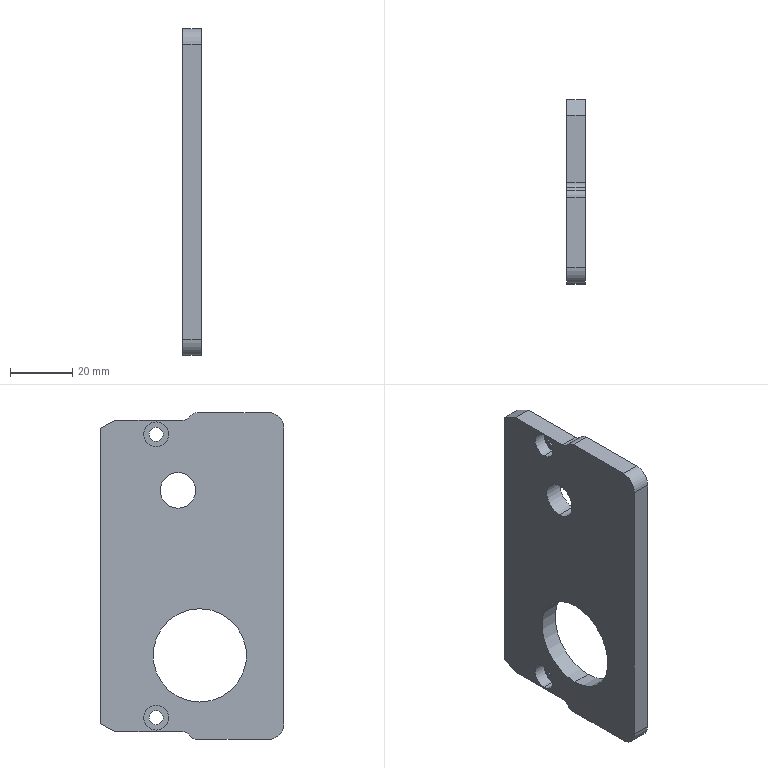Part | SolidWorks | features BaseBody 1 | 1 solid | 32 faces | box 6 x 59 x 105 mm | volume 30844 mm3 | cylinder 18 | plane 14 | commonest cylinder face diameters 4.5 x4 8 x4 5 x3 10 x2 11.445 x2 30 x2
STEP:
#1=CARTESIAN_POINT('',(-288.521,1920.544,-115.75));
#2=VERTEX_POINT('',#1);
#3=CARTESIAN_POINT('',(-288.521,1920.544,-120.25));
#4=VERTEX_POINT('',#3);
#5=CARTESIAN_POINT('',(-288.521,1920.544,-118.));
#6=DIRECTION('',(1.,0.,0.));
#7=DIRECTION('',(0.,0.,1.));
#8=AXIS2_PLACEMENT_3D('',#5,#6,#7);
#9=CIRCLE('',#8,2.25);
#10=EDGE_CURVE('',#2,#4,#9,.T.);
#11=ORIENTED_EDGE('',*,*,#10,.T.);
#12=CARTESIAN_POINT('',(-290.521,1920.544,-120.25));
#13=VERTEX_POINT('',#12);
#14=CARTESIAN_POINT('',(-173.931,1920.544,-120.25));
#15=DIRECTION('',(-1.,0.,0.));
#16=VECTOR('',#15,1000.);
#17=LINE('',#14,#16);
#18=EDGE_CURVE('',#4,#13,#17,.T.);
#19=ORIENTED_EDGE('',*,*,#18,.T.);
#20=CARTESIAN_POINT('',(-290.521,1920.544,-115.75));
#21=VERTEX_POINT('',#20);
#22=CARTESIAN_POINT('',(-290.521,1920.544,-118.));
#23=DIRECTION('',(1.,0.,0.));
#24=DIRECTION('',(0.,0.,1.));
#25=AXIS2_PLACEMENT_3D('',#22,#23,#24);
#26=CIRCLE('',#25,2.25);
#27=EDGE_CURVE('',#21,#13,#26,.T.);
#28=ORIENTED_EDGE('',*,*,#27,.F.);
#29=CARTESIAN_POINT('',(-173.931,1920.544,-115.75));
#30=DIRECTION('',(-1.,0.,0.));
#31=VECTOR('',#30,1000.);
#32=LINE('',#29,#31);
#33=EDGE_CURVE('',#2,#21,#32,.T.);
#34=ORIENTED_EDGE('',*,*,#33,.F.);
#35=EDGE_LOOP('',(#11,#19,#28,#34));
#36=FACE_OUTER_BOUND('',#35,.T.);
#37=CARTESIAN_POINT('',(-173.931,1920.544,-118.));
#38=DIRECTION('',(-1.,0.,0.));
#39=DIRECTION('',(0.,0.,1.));
#40=AXIS2_PLACEMENT_3D('',#37,#38,#39);
#41=CYLINDRICAL_SURFACE('',#40,2.25);
#42=ADVANCED_FACE('',(#36),#41,.F.);
#43=CARTESIAN_POINT('',(-288.521,1913.544,-39.278));
#44=VERTEX_POINT('',#43);
#45=CARTESIAN_POINT('',(-288.521,1913.544,-50.723));
#46=VERTEX_POINT('',#45);
#47=CARTESIAN_POINT('',(-288.521,1913.544,-45.));
#48=DIRECTION('',(1.,0.,0.));
#49=DIRECTION('',(0.,0.,1.));
#50=AXIS2_PLACEMENT_3D('',#47,#48,#49);
#51=CIRCLE('',#50,5.722);
#52=EDGE_CURVE('',#44,#46,#51,.T.);
#53=ORIENTED_EDGE('',*,*,#52,.T.);
#54=CARTESIAN_POINT('',(-294.521,1913.544,-50.723));
#55=VERTEX_POINT('',#54);
#56=CARTESIAN_POINT('',(-290.521,1913.544,-50.723));
#57=DIRECTION('',(-1.,0.,0.));
#58=VECTOR('',#57,1000.);
#59=LINE('',#56,#58);
#60=EDGE_CURVE('',#46,#55,#59,.T.);
#61=ORIENTED_EDGE('',*,*,#60,.T.);
#62=CARTESIAN_POINT('',(-294.521,1913.544,-39.278));
#63=VERTEX_POINT('',#62);
#64=CARTESIAN_POINT('',(-294.521,1913.544,-45.));
#65=DIRECTION('',(1.,0.,0.));
#66=DIRECTION('',(0.,0.,1.));
#67=AXIS2_PLACEMENT_3D('',#64,#65,#66);
#68=CIRCLE('',#67,5.722);
#69=EDGE_CURVE('',#63,#55,#68,.T.);
#70=ORIENTED_EDGE('',*,*,#69,.F.);
#71=CARTESIAN_POINT('',(-290.521,1913.544,-39.278));
#72=DIRECTION('',(-1.,0.,0.));
#73=VECTOR('',#72,1000.);
#74=LINE('',#71,#73);
#75=EDGE_CURVE('',#44,#63,#74,.T.);
#76=ORIENTED_EDGE('',*,*,#75,.F.);
#77=EDGE_LOOP('',(#53,#61,#70,#76));
#78=FACE_OUTER_BOUND('',#77,.T.);
#79=CARTESIAN_POINT('',(-290.521,1913.544,-45.));
#80=DIRECTION('',(-1.,0.,0.));
#81=DIRECTION('',(0.,0.,1.));
#82=AXIS2_PLACEMENT_3D('',#79,#80,#81);
#83=CYLINDRICAL_SURFACE('',#82,5.722);
#84=ADVANCED_FACE('',(#78),#83,.F.);
#85=CARTESIAN_POINT('',(-288.521,1906.544,-83.));
#86=VERTEX_POINT('',#85);
#87=CARTESIAN_POINT('',(-288.521,1906.544,-113.));
#88=VERTEX_POINT('',#87);
#89=CARTESIAN_POINT('',(-288.521,1906.544,-98.));
#90=DIRECTION('',(1.,0.,0.));
#91=DIRECTION('',(0.,0.,1.));
#92=AXIS2_PLACEMENT_3D('',#89,#90,#91);
#93=CIRCLE('',#92,15.);
#94=EDGE_CURVE('',#86,#88,#93,.T.);
#95=ORIENTED_EDGE('',*,*,#94,.T.);
#96=CARTESIAN_POINT('',(-294.521,1906.544,-113.));
#97=VERTEX_POINT('',#96);
#98=CARTESIAN_POINT('',(-173.931,1906.544,-113.));
#99=DIRECTION('',(-1.,0.,0.));
#100=VECTOR('',#99,1000.);
#101=LINE('',#98,#100);
#102=EDGE_CURVE('',#88,#97,#101,.T.);
#103=ORIENTED_EDGE('',*,*,#102,.T.);
#104=CARTESIAN_POINT('',(-294.521,1906.544,-83.));
#105=VERTEX_POINT('',#104);
#106=CARTESIAN_POINT('',(-294.521,1906.544,-98.));
#107=DIRECTION('',(1.,0.,0.));
#108=DIRECTION('',(0.,0.,1.));
#109=AXIS2_PLACEMENT_3D('',#106,#107,#108);
#110=CIRCLE('',#109,15.);
#111=EDGE_CURVE('',#105,#97,#110,.T.);
#112=ORIENTED_EDGE('',*,*,#111,.F.);
#113=CARTESIAN_POINT('',(-173.931,1906.544,-83.));
#114=DIRECTION('',(-1.,0.,0.));
#115=VECTOR('',#114,1000.);
#116=LINE('',#113,#115);
#117=EDGE_CURVE('',#86,#105,#116,.T.);
#118=ORIENTED_EDGE('',*,*,#117,.F.);
#119=EDGE_LOOP('',(#95,#103,#112,#118));
#120=FACE_OUTER_BOUND('',#119,.T.);
#121=CARTESIAN_POINT('',(-173.931,1906.544,-98.));
#122=DIRECTION('',(-1.,0.,0.));
#123=DIRECTION('',(0.,0.,1.));
#124=AXIS2_PLACEMENT_3D('',#121,#122,#123);
#125=CYLINDRICAL_SURFACE('',#124,15.);
#126=ADVANCED_FACE('',(#120),#125,.F.);
#127=CARTESIAN_POINT('',(-288.521,1920.544,-24.75));
#128=VERTEX_POINT('',#127);
#129=CARTESIAN_POINT('',(-288.521,1920.544,-29.25));
#130=VERTEX_POINT('',#129);
#131=CARTESIAN_POINT('',(-288.521,1920.544,-27.));
#132=DIRECTION('',(1.,0.,0.));
#133=DIRECTION('',(0.,0.,1.));
#134=AXIS2_PLACEMENT_3D('',#131,#132,#133);
#135=CIRCLE('',#134,2.25);
#136=EDGE_CURVE('',#128,#130,#135,.T.);
#137=ORIENTED_EDGE('',*,*,#136,.T.);
#138=CARTESIAN_POINT('',(-290.521,1920.544,-29.25));
#139=VERTEX_POINT('',#138);
#140=CARTESIAN_POINT('',(-173.931,1920.544,-29.25));
#141=DIRECTION('',(-1.,0.,0.));
#142=VECTOR('',#141,1000.);
#143=LINE('',#140,#142);
#144=EDGE_CURVE('',#130,#139,#143,.T.);
#145=ORIENTED_EDGE('',*,*,#144,.T.);
#146=CARTESIAN_POINT('',(-290.521,1920.544,-24.75));
#147=VERTEX_POINT('',#146);
#148=CARTESIAN_POINT('',(-290.521,1920.544,-27.));
#149=DIRECTION('',(1.,0.,0.));
#150=DIRECTION('',(0.,0.,1.));
#151=AXIS2_PLACEMENT_3D('',#148,#149,#150);
#152=CIRCLE('',#151,2.25);
#153=EDGE_CURVE('',#147,#139,#152,.T.);
#154=ORIENTED_EDGE('',*,*,#153,.F.);
#155=CARTESIAN_POINT('',(-173.931,1920.544,-24.75));
#156=DIRECTION('',(-1.,0.,0.));
#157=VECTOR('',#156,1000.);
#158=LINE('',#155,#157);
#159=EDGE_CURVE('',#128,#147,#158,.T.);
#160=ORIENTED_EDGE('',*,*,#159,.F.);
#161=EDGE_LOOP('',(#137,#145,#154,#160));
#162=FACE_OUTER_BOUND('',#161,.T.);
#163=CARTESIAN_POINT('',(-173.931,1920.544,-27.));
#164=DIRECTION('',(-1.,0.,0.));
#165=DIRECTION('',(0.,0.,1.));
#166=AXIS2_PLACEMENT_3D('',#163,#164,#165);
#167=CYLINDRICAL_SURFACE('',#166,2.25);
#168=ADVANCED_FACE('',(#162),#167,.F.);
#169=CARTESIAN_POINT('',(-290.521,1920.544,-122.));
#170=VERTEX_POINT('',#169);
#171=CARTESIAN_POINT('',(-290.521,1920.544,-114.));
#172=VERTEX_POINT('',#171);
#173=CARTESIAN_POINT('',(-290.521,1920.544,-118.));
#174=DIRECTION('',(-1.,0.,0.));
#175=DIRECTION('',(0.,0.,1.));
#176=AXIS2_PLACEMENT_3D('',#173,#174,#175);
#177=CIRCLE('',#176,4.);
#178=EDGE_CURVE('',#170,#172,#177,.T.);
#179=ORIENTED_EDGE('',*,*,#178,.F.);
#180=CARTESIAN_POINT('',(-294.521,1920.544,-122.));
#181=VERTEX_POINT('',#180);
#182=CARTESIAN_POINT('',(-292.521,1920.544,-122.));
#183=DIRECTION('',(-1.,0.,0.));
#184=VECTOR('',#183,1000.);
#185=LINE('',#182,#184);
#186=EDGE_CURVE('',#170,#181,#185,.T.);
#187=ORIENTED_EDGE('',*,*,#186,.T.);
#188=CARTESIAN_POINT('',(-294.521,1920.544,-114.));
#189=VERTEX_POINT('',#188);
#190=CARTESIAN_POINT('',(-294.521,1920.544,-118.));
#191=DIRECTION('',(1.,0.,0.));
#192=DIRECTION('',(0.,0.,1.));
#193=AXIS2_PLACEMENT_3D('',#190,#191,#192);
#194=CIRCLE('',#193,4.);
#195=EDGE_CURVE('',#189,#181,#194,.T.);
#196=ORIENTED_EDGE('',*,*,#195,.F.);
#197=CARTESIAN_POINT('',(-292.521,1920.544,-114.));
#198=DIRECTION('',(-1.,0.,0.));
#199=VECTOR('',#198,1000.);
#200=LINE('',#197,#199);
#201=EDGE_CURVE('',#172,#189,#200,.T.);
#202=ORIENTED_EDGE('',*,*,#201,.F.);
#203=EDGE_LOOP('',(#179,#187,#196,#202));
#204=FACE_OUTER_BOUND('',#203,.T.);
#205=CARTESIAN_POINT('',(-292.521,1920.544,-118.));
#206=DIRECTION('',(-1.,0.,0.));
#207=DIRECTION('',(0.,0.,1.));
#208=AXIS2_PLACEMENT_3D('',#205,#206,#207);
#209=CYLINDRICAL_SURFACE('',#208,4.);
#210=ADVANCED_FACE('',(#204),#209,.F.);
#211=CARTESIAN_POINT('',(-290.521,1920.544,-31.));
#212=VERTEX_POINT('',#211);
#213=CARTESIAN_POINT('',(-290.521,1920.544,-23.));
#214=VERTEX_POINT('',#213);
#215=CARTESIAN_POINT('',(-290.521,1920.544,-27.));
#216=DIRECTION('',(-1.,0.,0.));
#217=DIRECTION('',(0.,0.,1.));
#218=AXIS2_PLACEMENT_3D('',#215,#216,#217);
#219=CIRCLE('',#218,4.);
#220=EDGE_CURVE('',#212,#214,#219,.T.);
#221=ORIENTED_EDGE('',*,*,#220,.F.);
#222=CARTESIAN_POINT('',(-294.521,1920.544,-31.));
#223=VERTEX_POINT('',#222);
#224=CARTESIAN_POINT('',(-292.521,1920.544,-31.));
#225=DIRECTION('',(-1.,0.,0.));
#226=VECTOR('',#225,1000.);
#227=LINE('',#224,#226);
#228=EDGE_CURVE('',#212,#223,#227,.T.);
#229=ORIENTED_EDGE('',*,*,#228,.T.);
#230=CARTESIAN_POINT('',(-294.521,1920.544,-23.));
#231=VERTEX_POINT('',#230);
#232=CARTESIAN_POINT('',(-294.521,1920.544,-27.));
#233=DIRECTION('',(1.,0.,0.));
#234=DIRECTION('',(0.,0.,1.));
#235=AXIS2_PLACEMENT_3D('',#232,#233,#234);
#236=CIRCLE('',#235,4.);
#237=EDGE_CURVE('',#231,#223,#236,.T.);
#238=ORIENTED_EDGE('',*,*,#237,.F.);
#239=CARTESIAN_POINT('',(-292.521,1920.544,-23.));
#240=DIRECTION('',(-1.,0.,0.));
#241=VECTOR('',#240,1000.);
#242=LINE('',#239,#241);
#243=EDGE_CURVE('',#214,#231,#242,.T.);
#244=ORIENTED_EDGE('',*,*,#243,.F.);
#245=EDGE_LOOP('',(#221,#229,#238,#244));
#246=FACE_OUTER_BOUND('',#245,.T.);
#247=CARTESIAN_POINT('',(-292.521,1920.544,-27.));
#248=DIRECTION('',(-1.,0.,0.));
#249=DIRECTION('',(0.,0.,1.));
#250=AXIS2_PLACEMENT_3D('',#247,#248,#249);
#251=CYLINDRICAL_SURFACE('',#250,4.);
#252=ADVANCED_FACE('',(#246),#251,.F.);
#253=ORIENTED_EDGE('',*,*,#10,.F.);
#254=CARTESIAN_POINT('',(-288.521,1920.544,-118.));
#255=DIRECTION('',(1.,0.,0.));
#256=DIRECTION('',(0.,0.,1.));
#257=AXIS2_PLACEMENT_3D('',#254,#255,#256);
#258=CIRCLE('',#257,2.25);
#259=EDGE_CURVE('',#4,#2,#258,.T.);
#260=ORIENTED_EDGE('',*,*,#259,.F.);
#261=EDGE_LOOP('',(#253,#260));
#262=FACE_BOUND('',#261,.T.);
#263=ORIENTED_EDGE('',*,*,#52,.F.);
#264=CARTESIAN_POINT('',(-288.521,1913.544,-45.));
#265=DIRECTION('',(1.,0.,0.));
#266=DIRECTION('',(0.,0.,1.));
#267=AXIS2_PLACEMENT_3D('',#264,#265,#266);
#268=CIRCLE('',#267,5.722);
#269=EDGE_CURVE('',#46,#44,#268,.T.);
#270=ORIENTED_EDGE('',*,*,#269,.F.);
#271=EDGE_LOOP('',(#263,#270));
#272=FACE_BOUND('',#271,.T.);
#273=ORIENTED_EDGE('',*,*,#94,.F.);
#274=CARTESIAN_POINT('',(-288.521,1906.544,-98.));
#275=DIRECTION('',(1.,0.,0.));
#276=DIRECTION('',(0.,0.,1.));
#277=AXIS2_PLACEMENT_3D('',#274,#275,#276);
#278=CIRCLE('',#277,15.);
#279=EDGE_CURVE('',#88,#86,#278,.T.);
#280=ORIENTED_EDGE('',*,*,#279,.F.);
#281=EDGE_LOOP('',(#273,#280));
#282=FACE_BOUND('',#281,.T.);
#283=ORIENTED_EDGE('',*,*,#136,.F.);
#284=CARTESIAN_POINT('',(-288.521,1920.544,-27.));
#285=DIRECTION('',(1.,0.,0.));
#286=DIRECTION('',(0.,0.,1.));
#287=AXIS2_PLACEMENT_3D('',#284,#285,#286);
#288=CIRCLE('',#287,2.25);
#289=EDGE_CURVE('',#130,#128,#288,.T.);
#290=ORIENTED_EDGE('',*,*,#289,.F.);
#291=EDGE_LOOP('',(#283,#290));
#292=FACE_BOUND('',#291,.T.);
#293=CARTESIAN_POINT('',(-288.521,1912.08,-22.5));
#294=VERTEX_POINT('',#293);
#295=CARTESIAN_POINT('',(-288.521,1933.544,-22.5));
#296=VERTEX_POINT('',#295);
#297=CARTESIAN_POINT('',(-288.521,1909.044,-22.5));
#298=DIRECTION('',(0.,1.,0.));
#299=VECTOR('',#298,1000.);
#300=LINE('',#297,#299);
#301=EDGE_CURVE('',#294,#296,#300,.T.);
#302=ORIENTED_EDGE('',*,*,#301,.F.);
#303=CARTESIAN_POINT('',(-288.521,1910.312,-21.768));
#304=VERTEX_POINT('',#303);
#305=CARTESIAN_POINT('',(-288.521,1912.08,-20.));
#306=DIRECTION('',(1.,0.,0.));
#307=DIRECTION('',(0.,0.,1.));
#308=AXIS2_PLACEMENT_3D('',#305,#306,#307);
#309=CIRCLE('',#308,2.5);
#310=EDGE_CURVE('',#304,#294,#309,.T.);
#311=ORIENTED_EDGE('',*,*,#310,.F.);
#312=CARTESIAN_POINT('',(-288.521,1909.423,-20.879));
#313=VERTEX_POINT('',#312);
#314=CARTESIAN_POINT('',(-288.521,1909.423,-20.879));
#315=DIRECTION('',(0.,0.7071,-0.7071));
#316=VECTOR('',#315,1000.);
#317=LINE('',#314,#316);
#318=EDGE_CURVE('',#313,#304,#317,.T.);
#319=ORIENTED_EDGE('',*,*,#318,.F.);
#320=CARTESIAN_POINT('',(-288.521,1907.301,-20.));
#321=VERTEX_POINT('',#320);
#322=CARTESIAN_POINT('',(-288.521,1907.301,-23.));
#323=DIRECTION('',(-1.,0.,0.));
#324=DIRECTION('',(0.,0.,1.));
#325=AXIS2_PLACEMENT_3D('',#322,#323,#324);
#326=CIRCLE('',#325,3.);
#327=EDGE_CURVE('',#321,#313,#326,.T.);
#328=ORIENTED_EDGE('',*,*,#327,.F.);
#329=CARTESIAN_POINT('',(-288.521,1884.544,-20.));
#330=VERTEX_POINT('',#329);
#331=CARTESIAN_POINT('',(-288.521,1909.044,-20.));
#332=DIRECTION('',(0.,1.,0.));
#333=VECTOR('',#332,1000.);
#334=LINE('',#331,#333);
#335=EDGE_CURVE('',#330,#321,#334,.T.);
#336=ORIENTED_EDGE('',*,*,#335,.F.);
#337=CARTESIAN_POINT('',(-288.521,1879.544,-25.));
#338=VERTEX_POINT('',#337);
#339=CARTESIAN_POINT('',(-288.521,1884.544,-25.));
#340=DIRECTION('',(-1.,0.,0.));
#341=DIRECTION('',(0.,0.,1.));
#342=AXIS2_PLACEMENT_3D('',#339,#340,#341);
#343=CIRCLE('',#342,5.);
#344=EDGE_CURVE('',#338,#330,#343,.T.);
#345=ORIENTED_EDGE('',*,*,#344,.F.);
#346=CARTESIAN_POINT('',(-288.521,1879.544,-120.));
#347=VERTEX_POINT('',#346);
#348=CARTESIAN_POINT('',(-288.521,1879.544,-72.5));
#349=DIRECTION('',(0.,0.,1.));
#350=VECTOR('',#349,1000.);
#351=LINE('',#348,#350);
#352=EDGE_CURVE('',#347,#338,#351,.T.);
#353=ORIENTED_EDGE('',*,*,#352,.F.);
#354=CARTESIAN_POINT('',(-288.521,1884.544,-125.));
#355=VERTEX_POINT('',#354);
#356=CARTESIAN_POINT('',(-288.521,1884.544,-120.));
#357=DIRECTION('',(-1.,0.,0.));
#358=DIRECTION('',(0.,0.,1.));
#359=AXIS2_PLACEMENT_3D('',#356,#357,#358);
#360=CIRCLE('',#359,5.);
#361=EDGE_CURVE('',#355,#347,#360,.T.);
#362=ORIENTED_EDGE('',*,*,#361,.F.);
#363=CARTESIAN_POINT('',(-288.521,1907.508,-125.));
#364=VERTEX_POINT('',#363);
#365=CARTESIAN_POINT('',(-288.521,1909.044,-125.));
#366=DIRECTION('',(0.,-1.,0.));
#367=VECTOR('',#366,1000.);
#368=LINE('',#365,#367);
#369=EDGE_CURVE('',#364,#355,#368,.T.);
#370=ORIENTED_EDGE('',*,*,#369,.F.);
#371=CARTESIAN_POINT('',(-288.521,1909.276,-124.268));
#372=VERTEX_POINT('',#371);
#373=CARTESIAN_POINT('',(-288.521,1907.508,-122.5));
#374=DIRECTION('',(-1.,0.,0.));
#375=DIRECTION('',(0.,0.,-1.));
#376=AXIS2_PLACEMENT_3D('',#373,#374,#375);
#377=CIRCLE('',#376,2.5);
#378=EDGE_CURVE('',#372,#364,#377,.T.);
#379=ORIENTED_EDGE('',*,*,#378,.F.);
#380=CARTESIAN_POINT('',(-288.521,1910.312,-123.232));
#381=VERTEX_POINT('',#380);
#382=CARTESIAN_POINT('',(-288.521,1910.312,-123.232));
#383=DIRECTION('',(0.,-0.7071,-0.7071));
#384=VECTOR('',#383,1000.);
#385=LINE('',#382,#384);
#386=EDGE_CURVE('',#381,#372,#385,.T.);
#387=ORIENTED_EDGE('',*,*,#386,.F.);
#388=CARTESIAN_POINT('',(-288.521,1912.08,-122.5));
#389=VERTEX_POINT('',#388);
#390=CARTESIAN_POINT('',(-288.521,1912.08,-125.));
#391=DIRECTION('',(1.,0.,0.));
#392=DIRECTION('',(0.,0.,-1.));
#393=AXIS2_PLACEMENT_3D('',#390,#391,#392);
#394=CIRCLE('',#393,2.5);
#395=EDGE_CURVE('',#389,#381,#394,.T.);
#396=ORIENTED_EDGE('',*,*,#395,.F.);
#397=CARTESIAN_POINT('',(-288.521,1933.544,-122.5));
#398=VERTEX_POINT('',#397);
#399=CARTESIAN_POINT('',(-288.521,1909.044,-122.5));
#400=DIRECTION('',(0.,-1.,0.));
#401=VECTOR('',#400,1000.);
#402=LINE('',#399,#401);
#403=EDGE_CURVE('',#398,#389,#402,.T.);
#404=ORIENTED_EDGE('',*,*,#403,.F.);
#405=CARTESIAN_POINT('',(-288.521,1938.544,-120.));
#406=VERTEX_POINT('',#405);
#407=CARTESIAN_POINT('',(-288.521,1938.544,-120.));
#408=DIRECTION('',(0.,-0.8944,-0.4472));
#409=VECTOR('',#408,1000.);
#410=LINE('',#407,#409);
#411=EDGE_CURVE('',#406,#398,#410,.T.);
#412=ORIENTED_EDGE('',*,*,#411,.F.);
#413=CARTESIAN_POINT('',(-288.521,1938.544,-25.));
#414=VERTEX_POINT('',#413);
#415=CARTESIAN_POINT('',(-288.521,1938.544,-72.5));
#416=DIRECTION('',(0.,0.,-1.));
#417=VECTOR('',#416,1000.);
#418=LINE('',#415,#417);
#419=EDGE_CURVE('',#414,#406,#418,.T.);
#420=ORIENTED_EDGE('',*,*,#419,.F.);
#421=CARTESIAN_POINT('',(-288.521,1933.544,-22.5));
#422=DIRECTION('',(0.,0.8944,-0.4472));
#423=VECTOR('',#422,1000.);
#424=LINE('',#421,#423);
#425=EDGE_CURVE('',#296,#414,#424,.T.);
#426=ORIENTED_EDGE('',*,*,#425,.F.);
#427=EDGE_LOOP('',(#302,#311,#319,#328,#336,#345,#353,#362,#370,#379,#387,#396,#404,#412,#420,#426));
#428=FACE_OUTER_BOUND('',#427,.T.);
#429=CARTESIAN_POINT('',(-288.521,1909.044,-72.5));
#430=DIRECTION('',(-1.,0.,0.));
#431=DIRECTION('',(0.,0.,1.));
#432=AXIS2_PLACEMENT_3D('',#429,#430,#431);
#433=PLANE('',#432);
#434=ADVANCED_FACE('',(#262,#272,#282,#292,#428),#433,.F.);
#435=ORIENTED_EDGE('',*,*,#18,.F.);
#436=ORIENTED_EDGE('',*,*,#259,.T.);
#437=ORIENTED_EDGE('',*,*,#33,.T.);
#438=CARTESIAN_POINT('',(-290.521,1920.544,-118.));
#439=DIRECTION('',(1.,0.,0.));
#440=DIRECTION('',(0.,0.,1.));
#441=AXIS2_PLACEMENT_3D('',#438,#439,#440);
#442=CIRCLE('',#441,2.25);
#443=EDGE_CURVE('',#13,#21,#442,.T.);
#444=ORIENTED_EDGE('',*,*,#443,.F.);
#445=EDGE_LOOP('',(#435,#436,#437,#444));
#446=FACE_OUTER_BOUND('',#445,.T.);
#447=CARTESIAN_POINT('',(-173.931,1920.544,-118.));
#448=DIRECTION('',(-1.,0.,0.));
#449=DIRECTION('',(0.,0.,1.));
#450=AXIS2_PLACEMENT_3D('',#447,#448,#449);
#451=CYLINDRICAL_SURFACE('',#450,2.25);
#452=ADVANCED_FACE('',(#446),#451,.F.);
#453=ORIENTED_EDGE('',*,*,#60,.F.);
#454=ORIENTED_EDGE('',*,*,#269,.T.);
#455=ORIENTED_EDGE('',*,*,#75,.T.);
#456=CARTESIAN_POINT('',(-294.521,1913.544,-45.));
#457=DIRECTION('',(1.,0.,0.));
#458=DIRECTION('',(0.,0.,1.));
#459=AXIS2_PLACEMENT_3D('',#456,#457,#458);
#460=CIRCLE('',#459,5.722);
#461=EDGE_CURVE('',#55,#63,#460,.T.);
#462=ORIENTED_EDGE('',*,*,#461,.F.);
#463=EDGE_LOOP('',(#453,#454,#455,#462));
#464=FACE_OUTER_BOUND('',#463,.T.);
#465=CARTESIAN_POINT('',(-290.521,1913.544,-45.));
#466=DIRECTION('',(-1.,0.,0.));
#467=DIRECTION('',(0.,0.,1.));
#468=AXIS2_PLACEMENT_3D('',#465,#466,#467);
#469=CYLINDRICAL_SURFACE('',#468,5.722);
#470=ADVANCED_FACE('',(#464),#469,.F.);
#471=ORIENTED_EDGE('',*,*,#102,.F.);
#472=ORIENTED_EDGE('',*,*,#279,.T.);
#473=ORIENTED_EDGE('',*,*,#117,.T.);
#474=CARTESIAN_POINT('',(-294.521,1906.544,-98.));
#475=DIRECTION('',(1.,0.,0.));
#476=DIRECTION('',(0.,0.,1.));
#477=AXIS2_PLACEMENT_3D('',#474,#475,#476);
#478=CIRCLE('',#477,15.);
#479=EDGE_CURVE('',#97,#105,#478,.T.);
#480=ORIENTED_EDGE('',*,*,#479,.F.);
#481=EDGE_LOOP('',(#471,#472,#473,#480));
#482=FACE_OUTER_BOUND('',#481,.T.);
#483=CARTESIAN_POINT('',(-173.931,1906.544,-98.));
#484=DIRECTION('',(-1.,0.,0.));
#485=DIRECTION('',(0.,0.,1.));
#486=AXIS2_PLACEMENT_3D('',#483,#484,#485);
#487=CYLINDRICAL_SURFACE('',#486,15.);
#488=ADVANCED_FACE('',(#482),#487,.F.);
#489=ORIENTED_EDGE('',*,*,#144,.F.);
#490=ORIENTED_EDGE('',*,*,#289,.T.);
#491=ORIENTED_EDGE('',*,*,#159,.T.);
#492=CARTESIAN_POINT('',(-290.521,1920.544,-27.));
#493=DIRECTION('',(1.,0.,0.));
#494=DIRECTION('',(0.,0.,1.));
#495=AXIS2_PLACEMENT_3D('',#492,#493,#494);
#496=CIRCLE('',#495,2.25);
#497=EDGE_CURVE('',#139,#147,#496,.T.);
#498=ORIENTED_EDGE('',*,*,#497,.F.);
#499=EDGE_LOOP('',(#489,#490,#491,#498));
#500=FACE_OUTER_BOUND('',#499,.T.);
#501=CARTESIAN_POINT('',(-173.931,1920.544,-27.));
#502=DIRECTION('',(-1.,0.,0.));
#503=DIRECTION('',(0.,0.,1.));
#504=AXIS2_PLACEMENT_3D('',#501,#502,#503);
#505=CYLINDRICAL_SURFACE('',#504,2.25);
#506=ADVANCED_FACE('',(#500),#505,.F.);
#507=CARTESIAN_POINT('',(-294.521,1938.544,-25.));
#508=VERTEX_POINT('',#507);
#509=CARTESIAN_POINT('',(-288.521,1938.544,-25.));
#510=DIRECTION('',(-1.,0.,0.));
#511=VECTOR('',#510,1000.);
#512=LINE('',#509,#511);
#513=EDGE_CURVE('',#414,#508,#512,.T.);
#514=ORIENTED_EDGE('',*,*,#513,.T.);
#515=CARTESIAN_POINT('',(-294.521,1933.544,-22.5));
#516=VERTEX_POINT('',#515);
#517=CARTESIAN_POINT('',(-294.521,1936.044,-23.75));
#518=DIRECTION('',(0.,-0.8944,0.4472));
#519=VECTOR('',#518,1000.);
#520=LINE('',#517,#519);
#521=EDGE_CURVE('',#508,#516,#520,.T.);
#522=ORIENTED_EDGE('',*,*,#521,.T.);
#523=CARTESIAN_POINT('',(-288.521,1933.544,-22.5));
#524=DIRECTION('',(1.,0.,0.));
#525=VECTOR('',#524,1000.);
#526=LINE('',#523,#525);
#527=EDGE_CURVE('',#516,#296,#526,.T.);
#528=ORIENTED_EDGE('',*,*,#527,.T.);
#529=ORIENTED_EDGE('',*,*,#425,.T.);
#530=EDGE_LOOP('',(#514,#522,#528,#529));
#531=FACE_OUTER_BOUND('',#530,.T.);
#532=CARTESIAN_POINT('',(-288.521,1936.044,-23.75));
#533=DIRECTION('',(0.,0.4472,0.8944));
#534=DIRECTION('',(0.,-0.8944,0.4472));
#535=AXIS2_PLACEMENT_3D('',#532,#533,#534);
#536=PLANE('',#535);
#537=ADVANCED_FACE('',(#531),#536,.T.);
#538=CARTESIAN_POINT('',(-294.521,1912.08,-22.5));
#539=VERTEX_POINT('',#538);
#540=CARTESIAN_POINT('',(-294.521,1938.544,-22.5));
#541=DIRECTION('',(0.,-1.,0.));
#542=VECTOR('',#541,1000.);
#543=LINE('',#540,#542);
#544=EDGE_CURVE('',#516,#539,#543,.T.);
#545=ORIENTED_EDGE('',*,*,#544,.T.);
#546=CARTESIAN_POINT('',(-288.521,1912.08,-22.5));
#547=DIRECTION('',(1.,0.,0.));
#548=VECTOR('',#547,1000.);
#549=LINE('',#546,#548);
#550=EDGE_CURVE('',#539,#294,#549,.T.);
#551=ORIENTED_EDGE('',*,*,#550,.T.);
#552=ORIENTED_EDGE('',*,*,#301,.T.);
#553=ORIENTED_EDGE('',*,*,#527,.F.);
#554=EDGE_LOOP('',(#545,#551,#552,#553));
#555=FACE_OUTER_BOUND('',#554,.T.);
#556=CARTESIAN_POINT('',(-288.521,1938.544,-22.5));
#557=DIRECTION('',(0.,0.,1.));
#558=DIRECTION('',(1.,0.,0.));
#559=AXIS2_PLACEMENT_3D('',#556,#557,#558);
#560=PLANE('',#559);
#561=ADVANCED_FACE('',(#555),#560,.T.);
#562=CARTESIAN_POINT('',(-294.521,1910.312,-21.768));
#563=VERTEX_POINT('',#562);
#564=CARTESIAN_POINT('',(-288.521,1910.312,-21.768));
#565=DIRECTION('',(-1.,0.,0.));
#566=VECTOR('',#565,1000.);
#567=LINE('',#564,#566);
#568=EDGE_CURVE('',#304,#563,#567,.T.);
#569=ORIENTED_EDGE('',*,*,#568,.F.);
#570=ORIENTED_EDGE('',*,*,#310,.T.);
#571=ORIENTED_EDGE('',*,*,#550,.F.);
#572=CARTESIAN_POINT('',(-294.521,1912.08,-20.));
#573=DIRECTION('',(1.,0.,0.));
#574=DIRECTION('',(0.,0.,1.));
#575=AXIS2_PLACEMENT_3D('',#572,#573,#574);
#576=CIRCLE('',#575,2.5);
#577=EDGE_CURVE('',#563,#539,#576,.T.);
#578=ORIENTED_EDGE('',*,*,#577,.F.);
#579=EDGE_LOOP('',(#569,#570,#571,#578));
#580=FACE_OUTER_BOUND('',#579,.T.);
#581=CARTESIAN_POINT('',(-288.521,1912.08,-20.));
#582=DIRECTION('',(-1.,0.,0.));
#583=DIRECTION('',(0.,0.,1.));
#584=AXIS2_PLACEMENT_3D('',#581,#582,#583);
#585=CYLINDRICAL_SURFACE('',#584,2.5);
#586=ADVANCED_FACE('',(#580),#585,.F.);
#587=ORIENTED_EDGE('',*,*,#318,.T.);
#588=ORIENTED_EDGE('',*,*,#568,.T.);
#589=CARTESIAN_POINT('',(-294.521,1909.423,-20.879));
#590=VERTEX_POINT('',#589);
#591=CARTESIAN_POINT('',(-294.521,1909.794,-21.25));
#592=DIRECTION('',(0.,-0.7071,0.7071));
#593=VECTOR('',#592,1000.);
#594=LINE('',#591,#593);
#595=EDGE_CURVE('',#563,#590,#594,.T.);
#596=ORIENTED_EDGE('',*,*,#595,.T.);
#597=CARTESIAN_POINT('',(-288.521,1909.423,-20.879));
#598=DIRECTION('',(1.,0.,0.));
#599=VECTOR('',#598,1000.);
#600=LINE('',#597,#599);
#601=EDGE_CURVE('',#590,#313,#600,.T.);
#602=ORIENTED_EDGE('',*,*,#601,.T.);
#603=EDGE_LOOP('',(#587,#588,#596,#602));
#604=FACE_OUTER_BOUND('',#603,.T.);
#605=CARTESIAN_POINT('',(-288.521,1909.794,-21.25));
#606=DIRECTION('',(0.,0.7071,0.7071));
#607=DIRECTION('',(0.,-0.7071,0.7071));
#608=AXIS2_PLACEMENT_3D('',#605,#606,#607);
#609=PLANE('',#608);
#610=ADVANCED_FACE('',(#604),#609,.T.);
#611=CARTESIAN_POINT('',(-294.521,1907.301,-20.));
#612=VERTEX_POINT('',#611);
#613=CARTESIAN_POINT('',(-288.521,1907.301,-20.));
#614=DIRECTION('',(1.,0.,0.));
#615=VECTOR('',#614,1000.);
#616=LINE('',#613,#615);
#617=EDGE_CURVE('',#612,#321,#616,.T.);
#618=ORIENTED_EDGE('',*,*,#617,.T.);
#619=ORIENTED_EDGE('',*,*,#327,.T.);
#620=ORIENTED_EDGE('',*,*,#601,.F.);
#621=CARTESIAN_POINT('',(-294.521,1907.301,-23.));
#622=DIRECTION('',(1.,0.,0.));
#623=DIRECTION('',(0.,0.,1.));
#624=AXIS2_PLACEMENT_3D('',#621,#622,#623);
#625=CIRCLE('',#624,3.);
#626=EDGE_CURVE('',#590,#612,#625,.T.);
#627=ORIENTED_EDGE('',*,*,#626,.T.);
#628=EDGE_LOOP('',(#618,#619,#620,#627));
#629=FACE_OUTER_BOUND('',#628,.T.);
#630=CARTESIAN_POINT('',(-288.521,1907.301,-23.));
#631=DIRECTION('',(-1.,0.,0.));
#632=DIRECTION('',(0.,0.,1.));
#633=AXIS2_PLACEMENT_3D('',#630,#631,#632);
#634=CYLINDRICAL_SURFACE('',#633,3.);
#635=ADVANCED_FACE('',(#629),#634,.T.);
#636=ORIENTED_EDGE('',*,*,#335,.T.);
#637=ORIENTED_EDGE('',*,*,#617,.F.);
#638=CARTESIAN_POINT('',(-294.521,1884.544,-20.));
#639=VERTEX_POINT('',#638);
#640=CARTESIAN_POINT('',(-294.521,1938.544,-20.));
#641=DIRECTION('',(0.,-1.,0.));
#642=VECTOR('',#641,1000.);
#643=LINE('',#640,#642);
#644=EDGE_CURVE('',#612,#639,#643,.T.);
#645=ORIENTED_EDGE('',*,*,#644,.T.);
#646=CARTESIAN_POINT('',(-288.521,1884.544,-20.));
#647=DIRECTION('',(1.,0.,0.));
#648=VECTOR('',#647,1000.);
#649=LINE('',#646,#648);
#650=EDGE_CURVE('',#639,#330,#649,.T.);
#651=ORIENTED_EDGE('',*,*,#650,.T.);
#652=EDGE_LOOP('',(#636,#637,#645,#651));
#653=FACE_OUTER_BOUND('',#652,.T.);
#654=CARTESIAN_POINT('',(-288.521,1938.544,-20.));
#655=DIRECTION('',(0.,0.,1.));
#656=DIRECTION('',(1.,0.,0.));
#657=AXIS2_PLACEMENT_3D('',#654,#655,#656);
#658=PLANE('',#657);
#659=ADVANCED_FACE('',(#653),#658,.T.);
#660=CARTESIAN_POINT('',(-294.521,1879.544,-25.));
#661=VERTEX_POINT('',#660);
#662=CARTESIAN_POINT('',(-288.521,1879.544,-25.));
#663=DIRECTION('',(1.,0.,0.));
#664=VECTOR('',#663,1000.);
#665=LINE('',#662,#664);
#666=EDGE_CURVE('',#661,#338,#665,.T.);
#667=ORIENTED_EDGE('',*,*,#666,.T.);
#668=ORIENTED_EDGE('',*,*,#344,.T.);
#669=ORIENTED_EDGE('',*,*,#650,.F.);
#670=CARTESIAN_POINT('',(-294.521,1884.544,-25.));
#671=DIRECTION('',(1.,0.,0.));
#672=DIRECTION('',(0.,0.,1.));
#673=AXIS2_PLACEMENT_3D('',#670,#671,#672);
#674=CIRCLE('',#673,5.);
#675=EDGE_CURVE('',#639,#661,#674,.T.);
#676=ORIENTED_EDGE('',*,*,#675,.T.);
#677=EDGE_LOOP('',(#667,#668,#669,#676));
#678=FACE_OUTER_BOUND('',#677,.T.);
#679=CARTESIAN_POINT('',(-288.521,1884.544,-25.));
#680=DIRECTION('',(-1.,0.,0.));
#681=DIRECTION('',(0.,0.,1.));
#682=AXIS2_PLACEMENT_3D('',#679,#680,#681);
#683=CYLINDRICAL_SURFACE('',#682,5.);
#684=ADVANCED_FACE('',(#678),#683,.T.);
#685=ORIENTED_EDGE('',*,*,#352,.T.);
#686=ORIENTED_EDGE('',*,*,#666,.F.);
#687=CARTESIAN_POINT('',(-294.521,1879.544,-120.));
#688=VERTEX_POINT('',#687);
#689=CARTESIAN_POINT('',(-294.521,1879.544,-20.));
#690=DIRECTION('',(0.,0.,-1.));
#691=VECTOR('',#690,1000.);
#692=LINE('',#689,#691);
#693=EDGE_CURVE('',#661,#688,#692,.T.);
#694=ORIENTED_EDGE('',*,*,#693,.T.);
#695=CARTESIAN_POINT('',(-288.521,1879.544,-120.));
#696=DIRECTION('',(1.,0.,0.));
#697=VECTOR('',#696,1000.);
#698=LINE('',#695,#697);
#699=EDGE_CURVE('',#688,#347,#698,.T.);
#700=ORIENTED_EDGE('',*,*,#699,.T.);
#701=EDGE_LOOP('',(#685,#686,#694,#700));
#702=FACE_OUTER_BOUND('',#701,.T.);
#703=CARTESIAN_POINT('',(-288.521,1879.544,-20.));
#704=DIRECTION('',(0.,-1.,0.));
#705=DIRECTION('',(0.,0.,-1.));
#706=AXIS2_PLACEMENT_3D('',#703,#704,#705);
#707=PLANE('',#706);
#708=ADVANCED_FACE('',(#702),#707,.T.);
#709=CARTESIAN_POINT('',(-294.521,1884.544,-125.));
#710=VERTEX_POINT('',#709);
#711=CARTESIAN_POINT('',(-288.521,1884.544,-125.));
#712=DIRECTION('',(1.,0.,0.));
#713=VECTOR('',#712,1000.);
#714=LINE('',#711,#713);
#715=EDGE_CURVE('',#710,#355,#714,.T.);
#716=ORIENTED_EDGE('',*,*,#715,.T.);
#717=ORIENTED_EDGE('',*,*,#361,.T.);
#718=ORIENTED_EDGE('',*,*,#699,.F.);
#719=CARTESIAN_POINT('',(-294.521,1884.544,-120.));
#720=DIRECTION('',(1.,0.,0.));
#721=DIRECTION('',(0.,0.,1.));
#722=AXIS2_PLACEMENT_3D('',#719,#720,#721);
#723=CIRCLE('',#722,5.);
#724=EDGE_CURVE('',#688,#710,#723,.T.);
#725=ORIENTED_EDGE('',*,*,#724,.T.);
#726=EDGE_LOOP('',(#716,#717,#718,#725));
#727=FACE_OUTER_BOUND('',#726,.T.);
#728=CARTESIAN_POINT('',(-288.521,1884.544,-120.));
#729=DIRECTION('',(-1.,0.,0.));
#730=DIRECTION('',(0.,0.,1.));
#731=AXIS2_PLACEMENT_3D('',#728,#729,#730);
#732=CYLINDRICAL_SURFACE('',#731,5.);
#733=ADVANCED_FACE('',(#727),#732,.T.);
#734=CARTESIAN_POINT('',(-294.521,1907.508,-125.));
#735=VERTEX_POINT('',#734);
#736=CARTESIAN_POINT('',(-294.521,1879.544,-125.));
#737=DIRECTION('',(0.,1.,0.));
#738=VECTOR('',#737,1000.);
#739=LINE('',#736,#738);
#740=EDGE_CURVE('',#710,#735,#739,.T.);
#741=ORIENTED_EDGE('',*,*,#740,.T.);
#742=CARTESIAN_POINT('',(-288.521,1907.508,-125.));
#743=DIRECTION('',(1.,0.,0.));
#744=VECTOR('',#743,1000.);
#745=LINE('',#742,#744);
#746=EDGE_CURVE('',#735,#364,#745,.T.);
#747=ORIENTED_EDGE('',*,*,#746,.T.);
#748=ORIENTED_EDGE('',*,*,#369,.T.);
#749=ORIENTED_EDGE('',*,*,#715,.F.);
#750=EDGE_LOOP('',(#741,#747,#748,#749));
#751=FACE_OUTER_BOUND('',#750,.T.);
#752=CARTESIAN_POINT('',(-288.521,1879.544,-125.));
#753=DIRECTION('',(0.,0.,-1.));
#754=DIRECTION('',(-1.,0.,0.));
#755=AXIS2_PLACEMENT_3D('',#752,#753,#754);
#756=PLANE('',#755);
#757=ADVANCED_FACE('',(#751),#756,.T.);
#758=ORIENTED_EDGE('',*,*,#746,.F.);
#759=CARTESIAN_POINT('',(-294.521,1909.276,-124.268));
#760=VERTEX_POINT('',#759);
#761=CARTESIAN_POINT('',(-294.521,1907.508,-122.5));
#762=DIRECTION('',(1.,0.,0.));
#763=DIRECTION('',(0.,0.,-1.));
#764=AXIS2_PLACEMENT_3D('',#761,#762,#763);
#765=CIRCLE('',#764,2.5);
#766=EDGE_CURVE('',#735,#760,#765,.T.);
#767=ORIENTED_EDGE('',*,*,#766,.T.);
#768=CARTESIAN_POINT('',(-288.521,1909.276,-124.268));
#769=DIRECTION('',(1.,0.,0.));
#770=VECTOR('',#769,1000.);
#771=LINE('',#768,#770);
#772=EDGE_CURVE('',#760,#372,#771,.T.);
#773=ORIENTED_EDGE('',*,*,#772,.T.);
#774=ORIENTED_EDGE('',*,*,#378,.T.);
#775=EDGE_LOOP('',(#758,#767,#773,#774));
#776=FACE_OUTER_BOUND('',#775,.T.);
#777=CARTESIAN_POINT('',(-288.521,1907.508,-122.5));
#778=DIRECTION('',(1.,0.,0.));
#779=DIRECTION('',(0.,0.,-1.));
#780=AXIS2_PLACEMENT_3D('',#777,#778,#779);
#781=CYLINDRICAL_SURFACE('',#780,2.5);
#782=ADVANCED_FACE('',(#776),#781,.T.);
#783=ORIENTED_EDGE('',*,*,#386,.T.);
#784=ORIENTED_EDGE('',*,*,#772,.F.);
#785=CARTESIAN_POINT('',(-294.521,1910.312,-123.232));
#786=VERTEX_POINT('',#785);
#787=CARTESIAN_POINT('',(-294.521,1909.794,-123.75));
#788=DIRECTION('',(0.,0.7071,0.7071));
#789=VECTOR('',#788,1000.);
#790=LINE('',#787,#789);
#791=EDGE_CURVE('',#760,#786,#790,.T.);
#792=ORIENTED_EDGE('',*,*,#791,.T.);
#793=CARTESIAN_POINT('',(-288.521,1910.312,-123.232));
#794=DIRECTION('',(1.,0.,0.));
#795=VECTOR('',#794,1000.);
#796=LINE('',#793,#795);
#797=EDGE_CURVE('',#786,#381,#796,.T.);
#798=ORIENTED_EDGE('',*,*,#797,.T.);
#799=EDGE_LOOP('',(#783,#784,#792,#798));
#800=FACE_OUTER_BOUND('',#799,.T.);
#801=CARTESIAN_POINT('',(-288.521,1909.794,-123.75));
#802=DIRECTION('',(0.,0.7071,-0.7071));
#803=DIRECTION('',(0.,0.7071,0.7071));
#804=AXIS2_PLACEMENT_3D('',#801,#802,#803);
#805=PLANE('',#804);
#806=ADVANCED_FACE('',(#800),#805,.T.);
#807=ORIENTED_EDGE('',*,*,#797,.F.);
#808=CARTESIAN_POINT('',(-294.521,1912.08,-122.5));
#809=VERTEX_POINT('',#808);
#810=CARTESIAN_POINT('',(-294.521,1912.08,-125.));
#811=DIRECTION('',(1.,0.,0.));
#812=DIRECTION('',(0.,0.,-1.));
#813=AXIS2_PLACEMENT_3D('',#810,#811,#812);
#814=CIRCLE('',#813,2.5);
#815=EDGE_CURVE('',#809,#786,#814,.T.);
#816=ORIENTED_EDGE('',*,*,#815,.F.);
#817=CARTESIAN_POINT('',(-288.521,1912.08,-122.5));
#818=DIRECTION('',(-1.,0.,0.));
#819=VECTOR('',#818,1000.);
#820=LINE('',#817,#819);
#821=EDGE_CURVE('',#389,#809,#820,.T.);
#822=ORIENTED_EDGE('',*,*,#821,.F.);
#823=ORIENTED_EDGE('',*,*,#395,.T.);
#824=EDGE_LOOP('',(#807,#816,#822,#823));
#825=FACE_OUTER_BOUND('',#824,.T.);
#826=CARTESIAN_POINT('',(-288.521,1912.08,-125.));
#827=DIRECTION('',(1.,0.,0.));
#828=DIRECTION('',(0.,0.,-1.));
#829=AXIS2_PLACEMENT_3D('',#826,#827,#828);
#830=CYLINDRICAL_SURFACE('',#829,2.5);
#831=ADVANCED_FACE('',(#825),#830,.F.);
#832=CARTESIAN_POINT('',(-294.521,1933.544,-122.5));
#833=VERTEX_POINT('',#832);
#834=CARTESIAN_POINT('',(-294.521,1938.544,-122.5));
#835=DIRECTION('',(0.,-1.,0.));
#836=VECTOR('',#835,1000.);
#837=LINE('',#834,#836);
#838=EDGE_CURVE('',#833,#809,#837,.T.);
#839=ORIENTED_EDGE('',*,*,#838,.F.);
#840=CARTESIAN_POINT('',(-288.521,1933.544,-122.5));
#841=DIRECTION('',(-1.,0.,0.));
#842=VECTOR('',#841,1000.);
#843=LINE('',#840,#842);
#844=EDGE_CURVE('',#398,#833,#843,.T.);
#845=ORIENTED_EDGE('',*,*,#844,.F.);
#846=ORIENTED_EDGE('',*,*,#403,.T.);
#847=ORIENTED_EDGE('',*,*,#821,.T.);
#848=EDGE_LOOP('',(#839,#845,#846,#847));
#849=FACE_OUTER_BOUND('',#848,.T.);
#850=CARTESIAN_POINT('',(-288.521,1938.544,-122.5));
#851=DIRECTION('',(0.,0.,1.));
#852=DIRECTION('',(1.,0.,0.));
#853=AXIS2_PLACEMENT_3D('',#850,#851,#852);
#854=PLANE('',#853);
#855=ADVANCED_FACE('',(#849),#854,.F.);
#856=CARTESIAN_POINT('',(-294.521,1938.544,-120.));
#857=VERTEX_POINT('',#856);
#858=CARTESIAN_POINT('',(-288.521,1938.544,-120.));
#859=DIRECTION('',(1.,0.,0.));
#860=VECTOR('',#859,1000.);
#861=LINE('',#858,#860);
#862=EDGE_CURVE('',#857,#406,#861,.T.);
#863=ORIENTED_EDGE('',*,*,#862,.T.);
#864=ORIENTED_EDGE('',*,*,#411,.T.);
#865=ORIENTED_EDGE('',*,*,#844,.T.);
#866=CARTESIAN_POINT('',(-294.521,1936.044,-121.25));
#867=DIRECTION('',(0.,0.8944,0.4472));
#868=VECTOR('',#867,1000.);
#869=LINE('',#866,#868);
#870=EDGE_CURVE('',#833,#857,#869,.T.);
#871=ORIENTED_EDGE('',*,*,#870,.T.);
#872=EDGE_LOOP('',(#863,#864,#865,#871));
#873=FACE_OUTER_BOUND('',#872,.T.);
#874=CARTESIAN_POINT('',(-288.521,1936.044,-121.25));
#875=DIRECTION('',(0.,0.4472,-0.8944));
#876=DIRECTION('',(0.,0.8944,0.4472));
#877=AXIS2_PLACEMENT_3D('',#874,#875,#876);
#878=PLANE('',#877);
#879=ADVANCED_FACE('',(#873),#878,.T.);
#880=CARTESIAN_POINT('',(-294.521,1938.544,-125.));
#881=DIRECTION('',(0.,0.,1.));
#882=VECTOR('',#881,1000.);
#883=LINE('',#880,#882);
#884=EDGE_CURVE('',#857,#508,#883,.T.);
#885=ORIENTED_EDGE('',*,*,#884,.T.);
#886=ORIENTED_EDGE('',*,*,#513,.F.);
#887=ORIENTED_EDGE('',*,*,#419,.T.);
#888=ORIENTED_EDGE('',*,*,#862,.F.);
#889=EDGE_LOOP('',(#885,#886,#887,#888));
#890=FACE_OUTER_BOUND('',#889,.T.);
#891=CARTESIAN_POINT('',(-288.521,1938.544,-125.));
#892=DIRECTION('',(0.,1.,0.));
#893=DIRECTION('',(0.,0.,1.));
#894=AXIS2_PLACEMENT_3D('',#891,#892,#893);
#895=PLANE('',#894);
#896=ADVANCED_FACE('',(#890),#895,.T.);
#897=ORIENTED_EDGE('',*,*,#27,.T.);
#898=ORIENTED_EDGE('',*,*,#443,.T.);
#899=EDGE_LOOP('',(#897,#898));
#900=FACE_BOUND('',#899,.T.);
#901=CARTESIAN_POINT('',(-290.521,1920.544,-118.));
#902=DIRECTION('',(-1.,0.,0.));
#903=DIRECTION('',(0.,0.,1.));
#904=AXIS2_PLACEMENT_3D('',#901,#902,#903);
#905=CIRCLE('',#904,4.);
#906=EDGE_CURVE('',#172,#170,#905,.T.);
#907=ORIENTED_EDGE('',*,*,#906,.T.);
#908=ORIENTED_EDGE('',*,*,#178,.T.);
#909=EDGE_LOOP('',(#907,#908));
#910=FACE_OUTER_BOUND('',#909,.T.);
#911=CARTESIAN_POINT('',(-290.521,1920.544,-118.));
#912=DIRECTION('',(-1.,0.,0.));
#913=DIRECTION('',(0.,0.,1.));
#914=AXIS2_PLACEMENT_3D('',#911,#912,#913);
#915=PLANE('',#914);
#916=ADVANCED_FACE('',(#900,#910),#915,.T.);
#917=ORIENTED_EDGE('',*,*,#195,.T.);
#918=CARTESIAN_POINT('',(-294.521,1920.544,-118.));
#919=DIRECTION('',(1.,0.,0.));
#920=DIRECTION('',(0.,0.,1.));
#921=AXIS2_PLACEMENT_3D('',#918,#919,#920);
#922=CIRCLE('',#921,4.);
#923=EDGE_CURVE('',#181,#189,#922,.T.);
#924=ORIENTED_EDGE('',*,*,#923,.T.);
#925=EDGE_LOOP('',(#917,#924));
#926=FACE_BOUND('',#925,.T.);
#927=ORIENTED_EDGE('',*,*,#69,.T.);
#928=ORIENTED_EDGE('',*,*,#461,.T.);
#929=EDGE_LOOP('',(#927,#928));
#930=FACE_BOUND('',#929,.T.);
#931=ORIENTED_EDGE('',*,*,#111,.T.);
#932=ORIENTED_EDGE('',*,*,#479,.T.);
#933=EDGE_LOOP('',(#931,#932));
#934=FACE_BOUND('',#933,.T.);
#935=ORIENTED_EDGE('',*,*,#237,.T.);
#936=CARTESIAN_POINT('',(-294.521,1920.544,-27.));
#937=DIRECTION('',(1.,0.,0.));
#938=DIRECTION('',(0.,0.,1.));
#939=AXIS2_PLACEMENT_3D('',#936,#937,#938);
#940=CIRCLE('',#939,4.);
#941=EDGE_CURVE('',#223,#231,#940,.T.);
#942=ORIENTED_EDGE('',*,*,#941,.T.);
#943=EDGE_LOOP('',(#935,#942));
#944=FACE_BOUND('',#943,.T.);
#945=ORIENTED_EDGE('',*,*,#544,.F.);
#946=ORIENTED_EDGE('',*,*,#521,.F.);
#947=ORIENTED_EDGE('',*,*,#884,.F.);
#948=ORIENTED_EDGE('',*,*,#870,.F.);
#949=ORIENTED_EDGE('',*,*,#838,.T.);
#950=ORIENTED_EDGE('',*,*,#815,.T.);
#951=ORIENTED_EDGE('',*,*,#791,.F.);
#952=ORIENTED_EDGE('',*,*,#766,.F.);
#953=ORIENTED_EDGE('',*,*,#740,.F.);
#954=ORIENTED_EDGE('',*,*,#724,.F.);
#955=ORIENTED_EDGE('',*,*,#693,.F.);
#956=ORIENTED_EDGE('',*,*,#675,.F.);
#957=ORIENTED_EDGE('',*,*,#644,.F.);
#958=ORIENTED_EDGE('',*,*,#626,.F.);
#959=ORIENTED_EDGE('',*,*,#595,.F.);
#960=ORIENTED_EDGE('',*,*,#577,.T.);
#961=EDGE_LOOP('',(#945,#946,#947,#948,#949,#950,#951,#952,#953,#954,#955,#956,#957,#958,#959,#960));
#962=FACE_OUTER_BOUND('',#961,.T.);
#963=CARTESIAN_POINT('',(-294.521,1909.044,-72.5));
#964=DIRECTION('',(-1.,0.,0.));
#965=DIRECTION('',(0.,0.,1.));
#966=AXIS2_PLACEMENT_3D('',#963,#964,#965);
#967=PLANE('',#966);
#968=ADVANCED_FACE('',(#926,#930,#934,#944,#962),#967,.T.);
#969=ORIENTED_EDGE('',*,*,#153,.T.);
#970=ORIENTED_EDGE('',*,*,#497,.T.);
#971=EDGE_LOOP('',(#969,#970));
#972=FACE_BOUND('',#971,.T.);
#973=CARTESIAN_POINT('',(-290.521,1920.544,-27.));
#974=DIRECTION('',(-1.,0.,0.));
#975=DIRECTION('',(0.,0.,1.));
#976=AXIS2_PLACEMENT_3D('',#973,#974,#975);
#977=CIRCLE('',#976,4.);
#978=EDGE_CURVE('',#214,#212,#977,.T.);
#979=ORIENTED_EDGE('',*,*,#978,.T.);
#980=ORIENTED_EDGE('',*,*,#220,.T.);
#981=EDGE_LOOP('',(#979,#980));
#982=FACE_OUTER_BOUND('',#981,.T.);
#983=CARTESIAN_POINT('',(-290.521,1920.544,-27.));
#984=DIRECTION('',(-1.,0.,0.));
#985=DIRECTION('',(0.,0.,1.));
#986=AXIS2_PLACEMENT_3D('',#983,#984,#985);
#987=PLANE('',#986);
#988=ADVANCED_FACE('',(#972,#982),#987,.T.);
#989=ORIENTED_EDGE('',*,*,#186,.F.);
#990=ORIENTED_EDGE('',*,*,#906,.F.);
#991=ORIENTED_EDGE('',*,*,#201,.T.);
#992=ORIENTED_EDGE('',*,*,#923,.F.);
#993=EDGE_LOOP('',(#989,#990,#991,#992));
#994=FACE_OUTER_BOUND('',#993,.T.);
#995=CARTESIAN_POINT('',(-292.521,1920.544,-118.));
#996=DIRECTION('',(-1.,0.,0.));
#997=DIRECTION('',(0.,0.,1.));
#998=AXIS2_PLACEMENT_3D('',#995,#996,#997);
#999=CYLINDRICAL_SURFACE('',#998,4.);
#1000=ADVANCED_FACE('',(#994),#999,.F.);
#1001=ORIENTED_EDGE('',*,*,#228,.F.);
#1002=ORIENTED_EDGE('',*,*,#978,.F.);
#1003=ORIENTED_EDGE('',*,*,#243,.T.);
#1004=ORIENTED_EDGE('',*,*,#941,.F.);
#1005=EDGE_LOOP('',(#1001,#1002,#1003,#1004));
#1006=FACE_OUTER_BOUND('',#1005,.T.);
#1007=CARTESIAN_POINT('',(-292.521,1920.544,-27.));
#1008=DIRECTION('',(-1.,0.,0.));
#1009=DIRECTION('',(0.,0.,1.));
#1010=AXIS2_PLACEMENT_3D('',#1007,#1008,#1009);
#1011=CYLINDRICAL_SURFACE('',#1010,4.);
#1012=ADVANCED_FACE('',(#1006),#1011,.F.);
#1013=CLOSED_SHELL('',(#42,#84,#126,#168,#210,#252,#434,#452,#470,#488,#506,#537,#561,#586,#610,#635,#659,#684,#708,#733,#757,#782,#806,#831,#855,#879,#896,#916,#968,#988,#1000,#1012));
#1014=MANIFOLD_SOLID_BREP('',#1013);
#1015=CARTESIAN_POINT('',(0.,0.,0.));
#1016=DIRECTION('',(0.,0.,1.));
#1017=DIRECTION('',(1.,0.,0.));
#1018=AXIS2_PLACEMENT_3D('',#1015,#1016,#1017);
#1019=(LENGTH_UNIT()NAMED_UNIT(*)SI_UNIT(.MILLI.,.METRE.));
#1020=UNCERTAINTY_MEASURE_WITH_UNIT(LENGTH_MEASURE(0.00001),#1019,'','');
#1021=(NAMED_UNIT(*)PLANE_ANGLE_UNIT()SI_UNIT($,.RADIAN.));
#1022=(NAMED_UNIT(*)SI_UNIT($,.STERADIAN.)SOLID_ANGLE_UNIT());
#1023=(GEOMETRIC_REPRESENTATION_CONTEXT(3)GLOBAL_UNCERTAINTY_ASSIGNED_CONTEXT((#1020))GLOBAL_UNIT_ASSIGNED_CONTEXT((#1019,#1021,#1022))REPRESENTATION_CONTEXT('',''));
#1024=ADVANCED_BREP_SHAPE_REPRESENTATION('',(#1014,#1018),#1023);